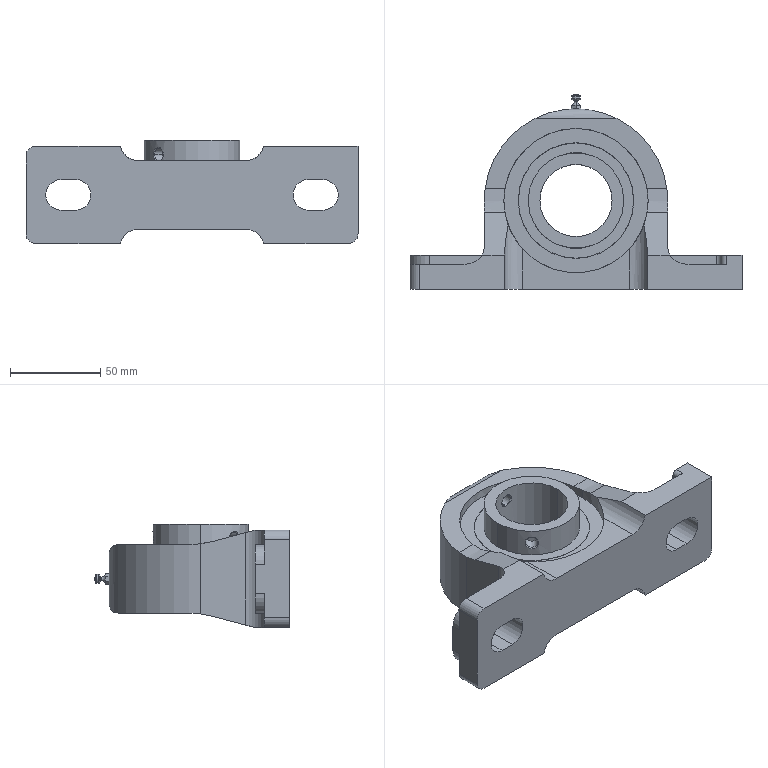Part | STEP file | Produce dryer line heating fan-UCP208_PDR40 | 1 solid | 113 faces | box 184 x 108 x 57.2 mm | volume 354732 mm3 | plane 46 | cylinder 41 | torus 16 | cone 10 | commonest cylinder face diameters 20.32 x6 101.6 x5 6.647 x4 17 x4 80 x4 10.8 x3